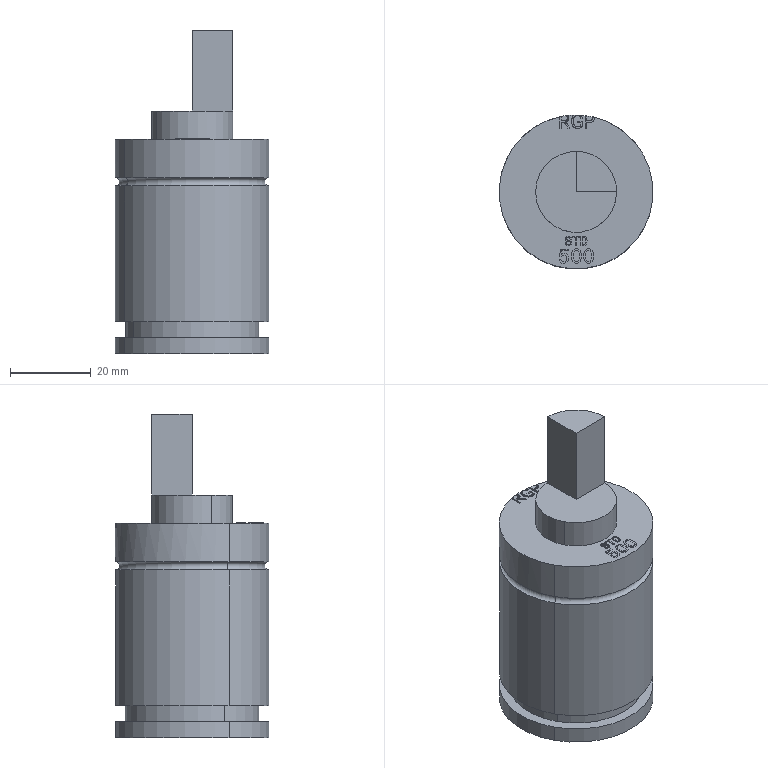Part | CATIA | 2 solids | 610 faces | box 38 x 38 x 80 mm | volume 62160 mm3 | plane 588 | cylinder 16 | cone 4 | torus 2 | commonest cylinder face diameters 38 x6 5 x4 20 x4 33 x2